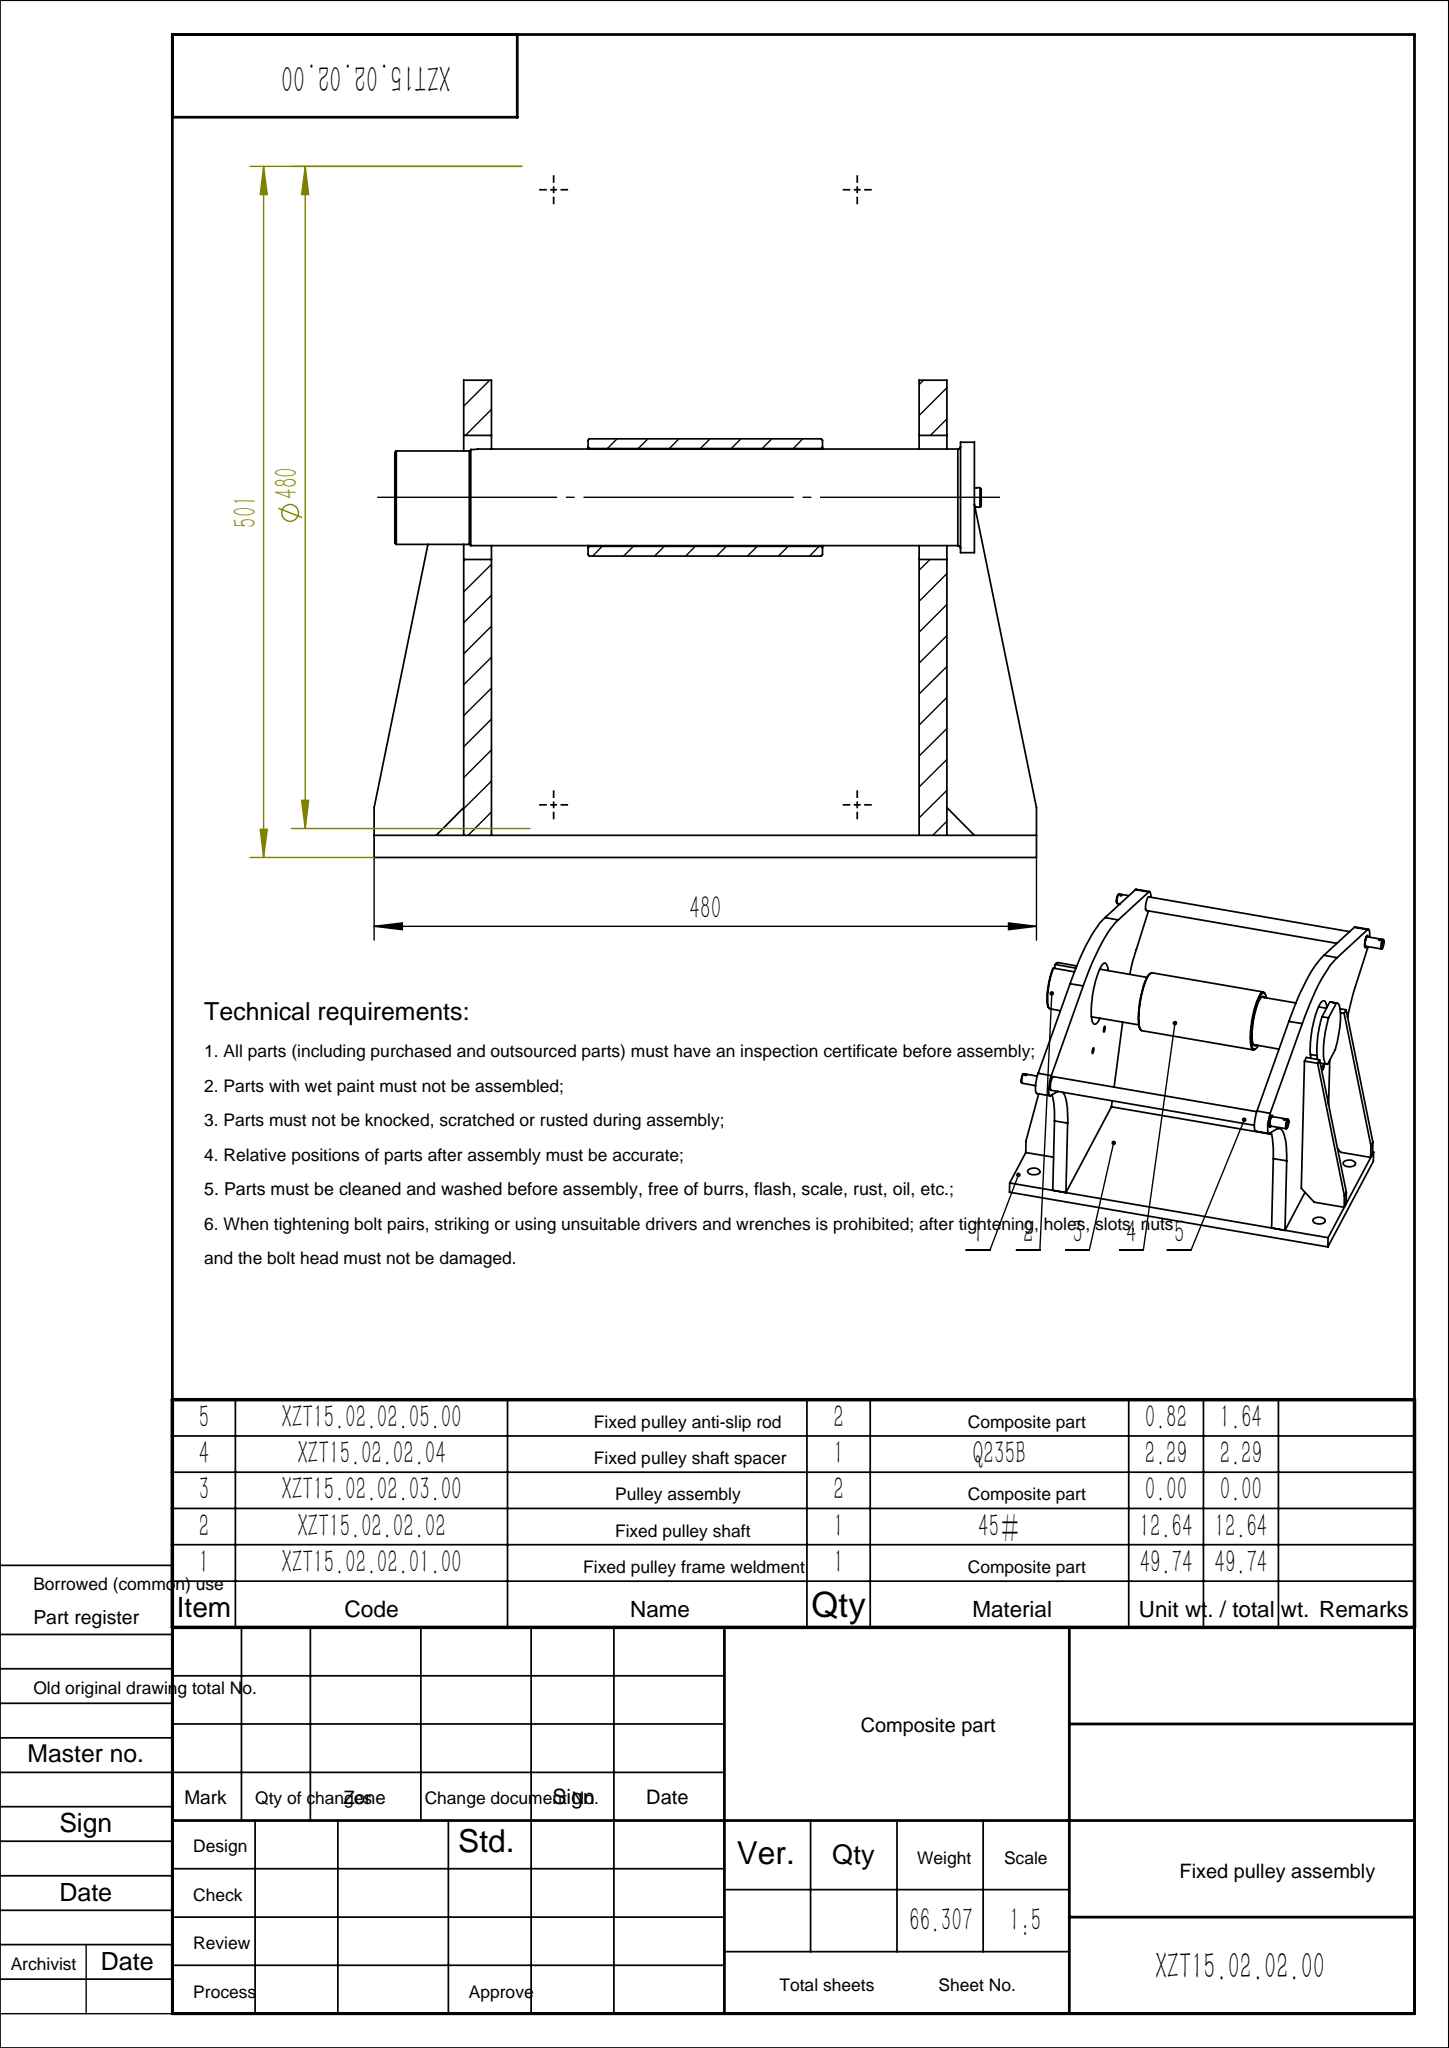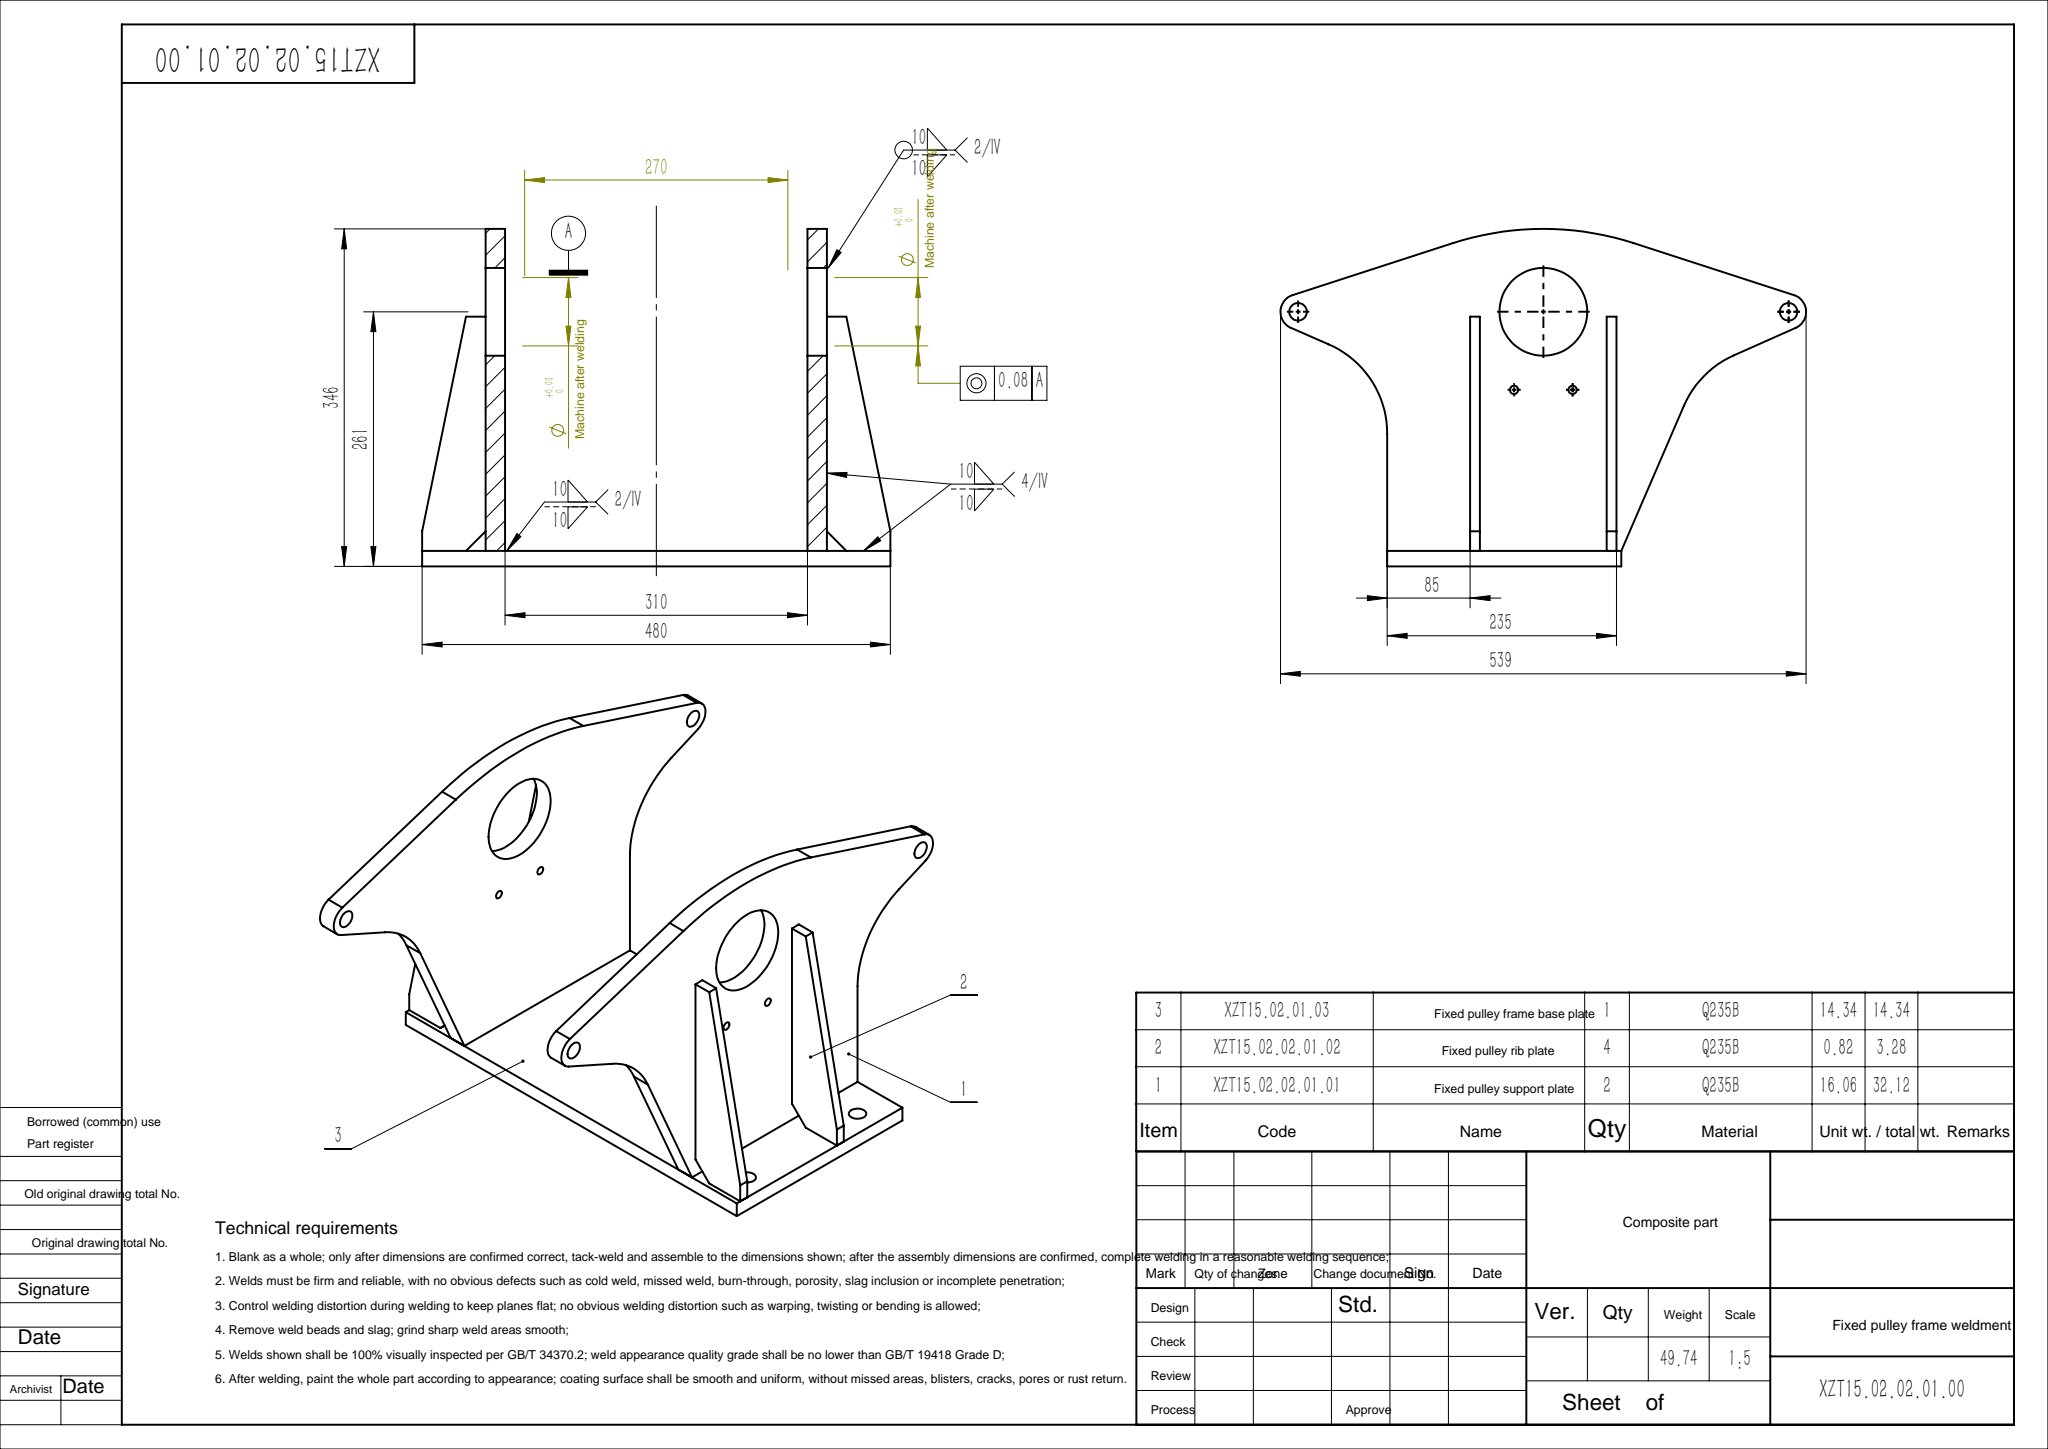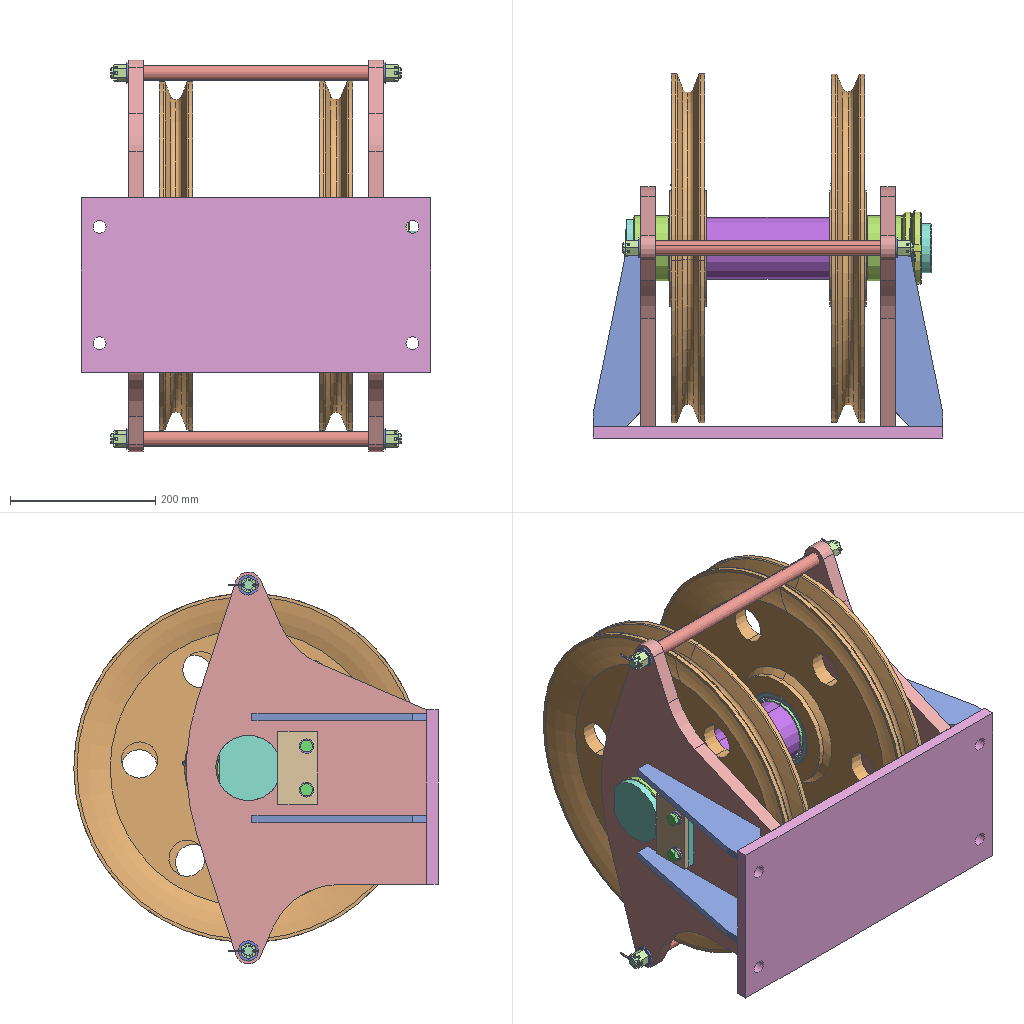Assembly | SolidWorks | 25 different items | 52 placed | box 480 x 501 x 539 mm
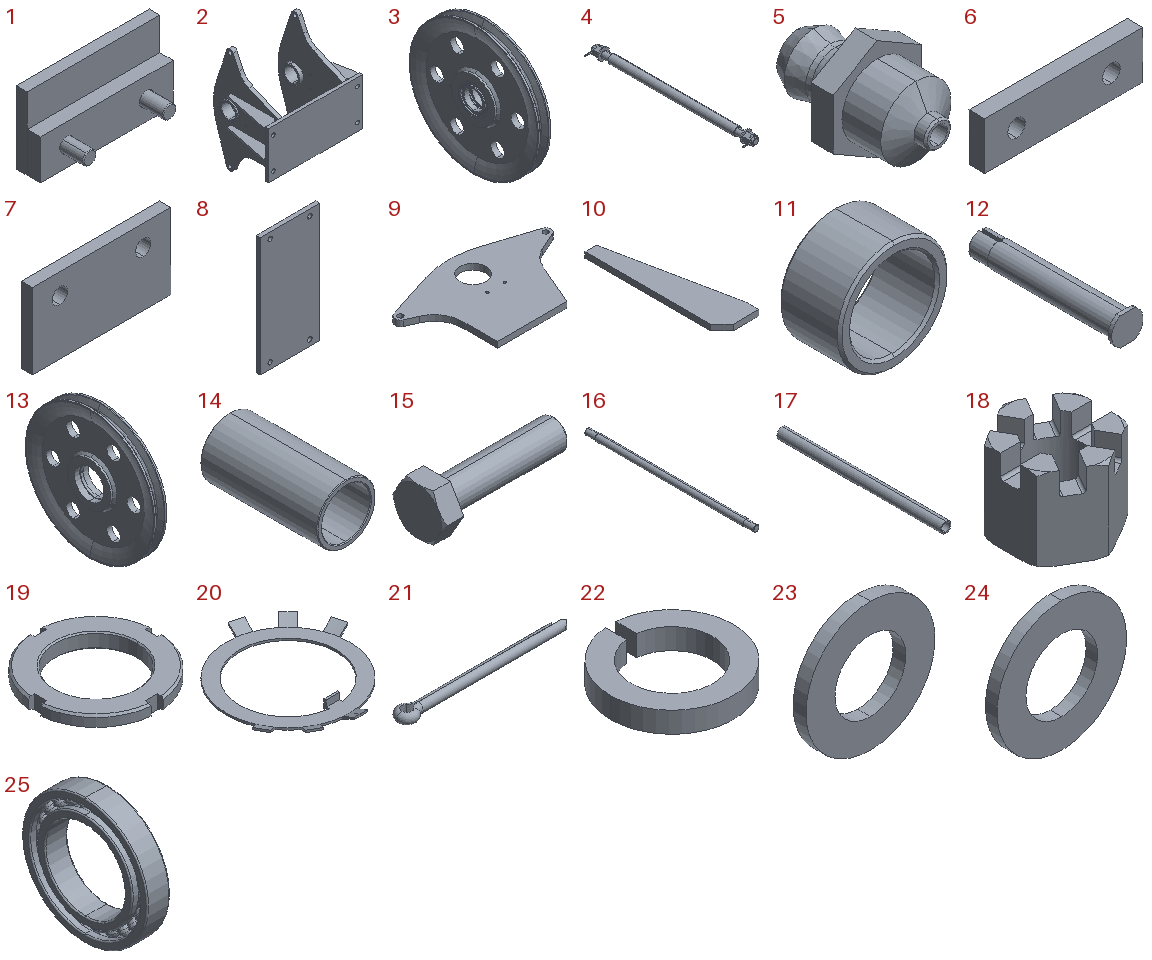Parts list (item | name | quantity | parent item | size | volume | features):
1 | (subassembly) | x1 | - | 100 x 46.4 x 54.5 mm | 80698 mm3 | features ReferencePattern 3, CompositeCurve 1, MirrorCompFeat 1
2 | (subassembly) | x1 | - | 480 x 346 x 539 mm | 6583524 mm3 | features ReferencePattern 4, MirrorCompFeat 1
3 | (subassembly) | x2 | - | 50 x 480 x 480 mm | 4092545 mm3 | features CompositeCurve 1
4 | (subassembly) | x2 | - | 41.5 x 400 x 28 mm | 113864 mm3 | features CompositeCurve 2
5 | - | x2 | in 3 | 10 x 16 x 11.547 mm | 627.343 mm3 | features Boss 1, Chamfer 1, Revolution 1
6 | - | x1 | in 1 | 100 x 10 x 30 mm | 28099 mm3 | features Extrusion 1, HoleWzd 1
7 | - | x1 | in 1 | 100 x 8 x 54.5 mm | 42079 mm3 | features Extrusion 1, HoleWzd 1
8 | - | x1 | in 2 | 240 x 16 x 480 mm | 1826914 mm3 | features Chamfer 1, Extrusion 1, Fillet 1, HoleWzd 1
9 | - | x2 | in 2 | 539 x 330 x 20 mm | 2045652 mm3 | features Extrusion 1, HoleWzd 1
10 | - | x4 | in 2 | 65 x 240 x 10 mm | 104500 mm3 | features Chamfer 1, Extrusion 1
11 | - | x2 | in 2 | 90 x 50 x 90 mm | 123653 mm3 | features Chamfer 1, Extrusion 1
12 | - | x1 | - | 90 x 420 x 80 mm | 1621053 mm3 | features Fillet 2, ICE 2, Chamfer 1, Revolution 1
13 | - | x2 | in 3 | 50 x 480 x 480 mm | 3922963 mm3 | features ICE 2, Chamfer 1, Fillet 1, MirrorPattern 1, RevCut 1, Revolution 1
14 | - | x1 | - | 85 x 170 x 85 mm | 291113 mm3 | features Chamfer 1, Extrusion 1
15 | - | x2 | in 1 | 46.4 x 18.475 x 16 mm | 4560 mm3 | features Chamfer 2, RevCut 2, Revolution 2, Extrusion 1, ICE 1
16 | - | x2 | in 4 | 15 x 400 x 15 mm | 69308 mm3 | features Chamfer 1, ICE 1, Revolution 1
17 | - | x2 | in 4 | 20 x 310 x 20 mm | 35060 mm3 | features WeldMemberFeat 1, WeldmentFeature 1
18 | - | x4 | in 4 | 19.728 x 22.78 x 17.8 mm | 3522 mm3 | features Cut 3, Chamfer 1, CirPattern 1, Extrusion 1
19 | - | x2 | - | 99.499 x 99.499 x 12 mm | 47793 mm3 | features Chamfer 3, CirPattern 1, Cut 1, Extrusion 1
20 | - | x1 | - | 99.417 x 104.021 x 6 mm | 4358 mm3 | features Boss 1, Cut 1, Revolution 1
21 | - | x4 | in 4 | 39.5 x 4.6 x 2.3 mm | 158.041 mm3 | features ICE 1, Sweep 1
22 | - | x2 | in 1 | 15.372 x 15.344 x 2.6 mm | 261.313 mm3 | features Extrusion 1
23 | - | x2 | in 1 | 20 x 2 x 20 mm | 438.252 mm3 | features Revolution 1
24 | - | x4 | in 4 | 28 x 2.5 x 28 mm | 1068 mm3 | features Revolution 1
25 | - | x4 | in 3 | 20 x 110 x 110 mm | 84477 mm3 | features Revolution 5, CirPattern 2, RefAxis 1, RevCut 1
Mates (type | each side: item.copy, entity, surface, feature):
In the top assembly
Concentric | 9.1 face cylinder Boss-Extrude1 | 17.1 face cylinder Gb/t 6728—2002 round tube 20 × 2(1)
Coincident | 24.1 face plane Base-Revolve | 24.2 face plane Base-Revolve
Concentric | 9.1 face cylinder Boss-Extrude1 | 16.1 face cylinder Revolve1
Coincident | 9.1 face plane Boss-Extrude1 | 24.1 face plane Base-Revolve
Parallel | 18.1 face plane Base-Extrude | 18.2 face plane Base-Extrude
Parallel | 8.1 face plane Boss-Extrude1 | 18.2 face plane Base-Extrude
Concentric | 11.1 face cylinder Boss-Extrude1 | 12.1 face cylinder Revolve1
Parallel | 8.1 face plane Boss-Extrude1 | 12.1 face plane Cut-Extrude1
Concentric | 12.1 face cylinder Revolve1 | 14.1 face cylinder Boss-Extrude1
Concentric | 12.1 face cylinder Revolve1 | 25.1 face cylinder Revolve1
Concentric | 12.1 face cylinder Revolve1 | 25.2 face cylinder Revolve1
Coincident | 25.3 face plane Revolve1 | 14.1 face plane Boss-Extrude1
Coincident | 11.1 face plane Boss-Extrude1 | 25.1 face plane Revolve1
Coincident | 14.1 face plane Boss-Extrude1 | 25.2 face plane Revolve1
Concentric | 19.1 face cylinder Base-Extrude | 19.2 face cylinder Base-Extrude
Coincident | 19.1 face plane CirPattern1 | 19.2 face plane CirPattern1
Concentric | 20.1 face cylinder Cut-Extrude2 | 19.2 face cylinder Base-Extrude
Coincident | 20.1 face plane Base-Revolve | 19.2 face plane Base-Extrude
Parallel | 20.1 face plane Cut-Extrude2 | 19.2 face plane CirPattern1
Coincident | 20.1 face plane Base-Revolve | 19.1 face plane Base-Extrude
Concentric | 12.1 face cylinder Revolve1 | 19.2 face cylinder Base-Extrude
Parallel | 12.1 face plane Cut-Extrude2 | 19.1 edge
Parallel | 12.1 face plane Cut-Extrude2 | 19.1 face plane CirPattern1
Coincident | 9.2 face plane Boss-Extrude1 | 6.1 face plane Boss-Extrude1
Concentric | 9.2 face cylinder M10 Tapped Hole1 | 15.1 face cylinder Revolve1
Parallel | 8.1 face plane Boss-Extrude1 | 6.1 face plane Boss-Extrude1
Coincident | 11.1 face plane Boss-Extrude1 | 19.2 face plane Base-Extrude
Coincident | 11.2 face plane Boss-Extrude1 | 12.1 face plane Revolve1
In subassembly 2
Coincident | 8.2 face plane Boss-Extrude1 | 2.1 plane
Coincident | 8.2 plane | 2.1 plane | 2 times
Coincident | 9.3 face plane Boss-Extrude1 | 8.2 face plane Boss-Extrude1
Coincident | 9.3 edge | 8.2 face plane Boss-Extrude1
Concentric | 9.3 face cylinder Boss-Extrude1 | 11.3 face cylinder Boss-Extrude1
DistanceDim | 9.3 face plane Boss-Extrude1 | 9.4 face plane Boss-Extrude1
Coincident | 9.3 face plane Boss-Extrude1 | 10.1 face plane Boss-Extrude1
Coincident | 10.1 face plane Boss-Extrude1 | 8.2 face plane Boss-Extrude1
Coincident | 8.2 face plane Boss-Extrude1 | 10.2 face plane Boss-Extrude1
Coincident | 9.3 face plane Boss-Extrude1 | 10.2 face plane Boss-Extrude1
DistanceDim | 10.1 face plane Boss-Extrude1 | 8.2 face plane Boss-Extrude1
DistanceDim | 10.2 face plane Boss-Extrude1 | 8.2 face plane Boss-Extrude1
DistanceDim | 11.4 face plane Boss-Extrude1 | 11.3 face plane Boss-Extrude1
In subassembly 1
Coordinate | 6.2 select_type:25 | 1.1 select_type:11
Concentric | 6.2 face cylinder Ø11.0 (11) Diameter Hole1 | 7.1 face cylinder Ø11.0 (11) Diameter Hole1
Coincident | 6.2 face plane Boss-Extrude1 | 7.1 face plane Boss-Extrude1 | 2 times
Concentric | 15.2 face cylinder Revolve1 | 22.1 face cylinder Extrude1
Concentric | 15.2 face cylinder Revolve1 | 23.1 face cylinder Base-Revolve
Concentric | 7.1 face cylinder Ø11.0 (11) Diameter Hole1 | 15.2 face cylinder Revolve1
Coincident | 23.1 face plane Base-Revolve | 22.1 face plane Extrude1
Coincident | 15.2 face plane Boss-Extrude1 | 22.1 face plane Extrude1
Coincident | 7.1 face plane Boss-Extrude1 | 23.1 face plane Base-Revolve
Parallel | 7.1 face plane Boss-Extrude1 | 15.2 face plane Boss-Extrude1
In subassembly 3
Concentric | 13.1 face cylinder Cut-Extrude1 | 25.4 face cylinder Revolve1
Concentric | 13.1 face cylinder Mirror1 | 25.5 edge
Coincident | 13.1 face plane Cut-Extrude2 | 25.5 face plane Revolve1
Coincident | 13.1 face plane Mirror1 | 25.4 face plane Revolve1
Concentric | 13.1 face cylinder Cut-Revolve1 | 5.1 face cylinder Revolve2
Coincident | 13.1 edge | 5.1 face plane Revolve2
In subassembly 4
Coordinate | 16.2 select_type:25 | 4.1 select_type:11
Concentric | 18.3 face cylinder Base-Extrude | 24.3 face cylinder Base-Revolve
Coincident | 18.3 face plane Base-Extrude | 24.3 face plane Base-Revolve
Concentric | 16.2 face cylinder Revolve1 | 24.3 face cylinder Base-Revolve
Coincident | 16.2 face plane Revolve1 | 24.3 face plane Base-Revolve
Concentric | 24.4 face cylinder Base-Revolve | 18.4 face cylinder Base-Extrude
Coincident | 24.4 face plane Base-Revolve | 18.4 face plane Base-Extrude
Parallel | 18.3 face plane Base-Extrude | 18.4 face plane Base-Extrude
Concentric | 16.2 face cylinder Revolve1 | 24.4 face cylinder Base-Revolve
Coincident | 16.2 face plane Revolve1 | 24.4 face plane Base-Revolve
Parallel | 18.3 face plane Base-Extrude | 4.1 plane
Concentric | 16.2 face cylinder Cut-Extrude1 | 21.1 face cylinder Sweep2
Parallel | 24.3 face plane Base-Revolve | 21.1 face plane Sweep2
Tangent | 16.2 face cylinder Revolve1 | 21.1 edge
Concentric | 16.2 face cylinder Cut-Extrude1 | 21.2 face cylinder Sweep2
Tangent | 16.2 face cylinder Revolve1 | 21.2 edge
Parallel | 24.4 face plane Base-Revolve | 21.2 face plane Sweep2
Concentric | 16.2 face cylinder Revolve1 | 17.2 face cylinder Gb/t 6728—2002 round tube 20 × 2(1)
DistanceDim | 17.2 face plane Gb/t 6728—2002 round tube 20 × 2(1) | 24.3 face plane Base-Revolve